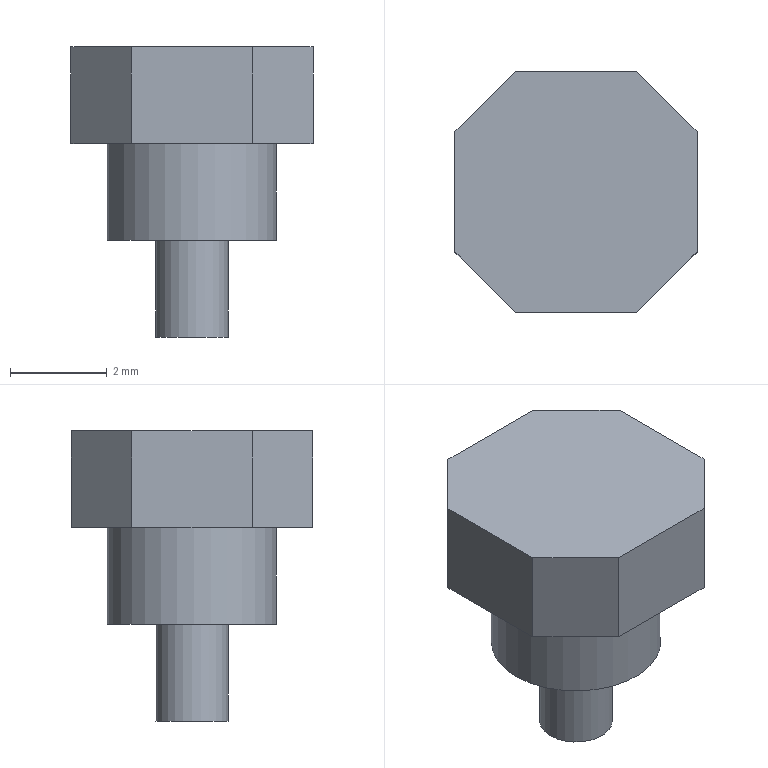Part | NX | features DATUM_CSYS 4, EXTRUDE 3, SKETCH 3, SYMBOLIC_THREAD 1 | 1 solid | 14 faces | box 5 x 4.979 x 6 mm | volume 66.325 mm3 | plane 12 | cylinder 2 | commonest cylinder face diameters 1.5 x1 3.5 x1
STEP:
#1=CARTESIAN_POINT('',(-1.251,-2.49,0.));
#2=VERTEX_POINT('',#1);
#3=CARTESIAN_POINT('',(1.251,-2.49,0.));
#4=VERTEX_POINT('',#3);
#5=CARTESIAN_POINT('',(-1.251,-2.49,0.));
#6=DIRECTION('',(1.,0.,0.));
#7=VECTOR('',#6,1000.);
#8=LINE('',#5,#7);
#9=EDGE_CURVE('',#2,#4,#8,.T.);
#10=ORIENTED_EDGE('',*,*,#9,.T.);
#11=CARTESIAN_POINT('',(1.251,-2.49,2.));
#12=VERTEX_POINT('',#11);
#13=CARTESIAN_POINT('',(1.251,-2.49,2.));
#14=DIRECTION('',(0.,0.,-1.));
#15=VECTOR('',#14,1000.);
#16=LINE('',#13,#15);
#17=EDGE_CURVE('',#12,#4,#16,.T.);
#18=ORIENTED_EDGE('',*,*,#17,.F.);
#19=CARTESIAN_POINT('',(-1.251,-2.49,2.));
#20=VERTEX_POINT('',#19);
#21=CARTESIAN_POINT('',(-1.251,-2.49,2.));
#22=DIRECTION('',(1.,0.,0.));
#23=VECTOR('',#22,1000.);
#24=LINE('',#21,#23);
#25=EDGE_CURVE('',#20,#12,#24,.T.);
#26=ORIENTED_EDGE('',*,*,#25,.F.);
#27=CARTESIAN_POINT('',(-1.251,-2.49,2.));
#28=DIRECTION('',(0.,0.,-1.));
#29=VECTOR('',#28,1000.);
#30=LINE('',#27,#29);
#31=EDGE_CURVE('',#20,#2,#30,.T.);
#32=ORIENTED_EDGE('',*,*,#31,.T.);
#33=EDGE_LOOP('',(#10,#18,#26,#32));
#34=FACE_BOUND('',#33,.T.);
#35=CARTESIAN_POINT('',(-1.251,-2.49,2.));
#36=DIRECTION('',(0.,1.,0.));
#37=DIRECTION('',(-1.,0.,0.));
#38=AXIS2_PLACEMENT_3D('',#35,#36,#37);
#39=PLANE('',#38);
#40=ADVANCED_FACE('',(#34),#39,.F.);
#41=CARTESIAN_POINT('',(2.5,-1.24,0.));
#42=VERTEX_POINT('',#41);
#43=CARTESIAN_POINT('',(1.251,-2.49,0.));
#44=DIRECTION('',(0.7071,0.7071,0.));
#45=VECTOR('',#44,1000.);
#46=LINE('',#43,#45);
#47=EDGE_CURVE('',#4,#42,#46,.T.);
#48=ORIENTED_EDGE('',*,*,#47,.T.);
#49=CARTESIAN_POINT('',(2.5,-1.24,2.));
#50=VERTEX_POINT('',#49);
#51=CARTESIAN_POINT('',(2.5,-1.24,2.));
#52=DIRECTION('',(0.,0.,-1.));
#53=VECTOR('',#52,1000.);
#54=LINE('',#51,#53);
#55=EDGE_CURVE('',#50,#42,#54,.T.);
#56=ORIENTED_EDGE('',*,*,#55,.F.);
#57=CARTESIAN_POINT('',(1.251,-2.49,2.));
#58=DIRECTION('',(0.7071,0.7071,0.));
#59=VECTOR('',#58,1000.);
#60=LINE('',#57,#59);
#61=EDGE_CURVE('',#12,#50,#60,.T.);
#62=ORIENTED_EDGE('',*,*,#61,.F.);
#63=ORIENTED_EDGE('',*,*,#17,.T.);
#64=EDGE_LOOP('',(#48,#56,#62,#63));
#65=FACE_BOUND('',#64,.T.);
#66=CARTESIAN_POINT('',(1.251,-2.49,2.));
#67=DIRECTION('',(-0.7071,0.7071,0.));
#68=DIRECTION('',(-0.7071,-0.7071,0.));
#69=AXIS2_PLACEMENT_3D('',#66,#67,#68);
#70=PLANE('',#69);
#71=ADVANCED_FACE('',(#65),#70,.F.);
#72=CARTESIAN_POINT('',(2.5,1.24,0.));
#73=VERTEX_POINT('',#72);
#74=CARTESIAN_POINT('',(2.5,-1.24,0.));
#75=DIRECTION('',(0.,1.,0.));
#76=VECTOR('',#75,1000.);
#77=LINE('',#74,#76);
#78=EDGE_CURVE('',#42,#73,#77,.T.);
#79=ORIENTED_EDGE('',*,*,#78,.T.);
#80=CARTESIAN_POINT('',(2.5,1.24,2.));
#81=VERTEX_POINT('',#80);
#82=CARTESIAN_POINT('',(2.5,1.24,2.));
#83=DIRECTION('',(0.,0.,-1.));
#84=VECTOR('',#83,1000.);
#85=LINE('',#82,#84);
#86=EDGE_CURVE('',#81,#73,#85,.T.);
#87=ORIENTED_EDGE('',*,*,#86,.F.);
#88=CARTESIAN_POINT('',(2.5,-1.24,2.));
#89=DIRECTION('',(0.,1.,0.));
#90=VECTOR('',#89,1000.);
#91=LINE('',#88,#90);
#92=EDGE_CURVE('',#50,#81,#91,.T.);
#93=ORIENTED_EDGE('',*,*,#92,.F.);
#94=ORIENTED_EDGE('',*,*,#55,.T.);
#95=EDGE_LOOP('',(#79,#87,#93,#94));
#96=FACE_BOUND('',#95,.T.);
#97=CARTESIAN_POINT('',(2.5,-1.24,2.));
#98=DIRECTION('',(-1.,0.,0.));
#99=DIRECTION('',(0.,0.,1.));
#100=AXIS2_PLACEMENT_3D('',#97,#98,#99);
#101=PLANE('',#100);
#102=ADVANCED_FACE('',(#96),#101,.F.);
#103=CARTESIAN_POINT('',(1.251,2.49,0.));
#104=VERTEX_POINT('',#103);
#105=CARTESIAN_POINT('',(2.5,1.24,0.));
#106=DIRECTION('',(-0.7071,0.7071,0.));
#107=VECTOR('',#106,1000.);
#108=LINE('',#105,#107);
#109=EDGE_CURVE('',#73,#104,#108,.T.);
#110=ORIENTED_EDGE('',*,*,#109,.T.);
#111=CARTESIAN_POINT('',(1.251,2.49,2.));
#112=VERTEX_POINT('',#111);
#113=CARTESIAN_POINT('',(1.251,2.49,2.));
#114=DIRECTION('',(0.,0.,-1.));
#115=VECTOR('',#114,1000.);
#116=LINE('',#113,#115);
#117=EDGE_CURVE('',#112,#104,#116,.T.);
#118=ORIENTED_EDGE('',*,*,#117,.F.);
#119=CARTESIAN_POINT('',(2.5,1.24,2.));
#120=DIRECTION('',(-0.7071,0.7071,0.));
#121=VECTOR('',#120,1000.);
#122=LINE('',#119,#121);
#123=EDGE_CURVE('',#81,#112,#122,.T.);
#124=ORIENTED_EDGE('',*,*,#123,.F.);
#125=ORIENTED_EDGE('',*,*,#86,.T.);
#126=EDGE_LOOP('',(#110,#118,#124,#125));
#127=FACE_BOUND('',#126,.T.);
#128=CARTESIAN_POINT('',(2.5,1.24,2.));
#129=DIRECTION('',(-0.7071,-0.7071,0.));
#130=DIRECTION('',(0.7071,-0.7071,0.));
#131=AXIS2_PLACEMENT_3D('',#128,#129,#130);
#132=PLANE('',#131);
#133=ADVANCED_FACE('',(#127),#132,.F.);
#134=CARTESIAN_POINT('',(-1.251,2.49,0.));
#135=VERTEX_POINT('',#134);
#136=CARTESIAN_POINT('',(1.251,2.49,0.));
#137=DIRECTION('',(-1.,0.,0.));
#138=VECTOR('',#137,1000.);
#139=LINE('',#136,#138);
#140=EDGE_CURVE('',#104,#135,#139,.T.);
#141=ORIENTED_EDGE('',*,*,#140,.T.);
#142=CARTESIAN_POINT('',(-1.251,2.49,2.));
#143=VERTEX_POINT('',#142);
#144=CARTESIAN_POINT('',(-1.251,2.49,2.));
#145=DIRECTION('',(0.,0.,-1.));
#146=VECTOR('',#145,1000.);
#147=LINE('',#144,#146);
#148=EDGE_CURVE('',#143,#135,#147,.T.);
#149=ORIENTED_EDGE('',*,*,#148,.F.);
#150=CARTESIAN_POINT('',(1.251,2.49,2.));
#151=DIRECTION('',(-1.,0.,0.));
#152=VECTOR('',#151,1000.);
#153=LINE('',#150,#152);
#154=EDGE_CURVE('',#112,#143,#153,.T.);
#155=ORIENTED_EDGE('',*,*,#154,.F.);
#156=ORIENTED_EDGE('',*,*,#117,.T.);
#157=EDGE_LOOP('',(#141,#149,#155,#156));
#158=FACE_BOUND('',#157,.T.);
#159=CARTESIAN_POINT('',(1.251,2.49,2.));
#160=DIRECTION('',(0.,-1.,0.));
#161=DIRECTION('',(0.,0.,-1.));
#162=AXIS2_PLACEMENT_3D('',#159,#160,#161);
#163=PLANE('',#162);
#164=ADVANCED_FACE('',(#158),#163,.F.);
#165=CARTESIAN_POINT('',(-2.5,1.24,0.));
#166=VERTEX_POINT('',#165);
#167=CARTESIAN_POINT('',(-1.251,2.49,0.));
#168=DIRECTION('',(-0.7071,-0.7071,0.));
#169=VECTOR('',#168,1000.);
#170=LINE('',#167,#169);
#171=EDGE_CURVE('',#135,#166,#170,.T.);
#172=ORIENTED_EDGE('',*,*,#171,.T.);
#173=CARTESIAN_POINT('',(-2.5,1.24,2.));
#174=VERTEX_POINT('',#173);
#175=CARTESIAN_POINT('',(-2.5,1.24,2.));
#176=DIRECTION('',(0.,0.,-1.));
#177=VECTOR('',#176,1000.);
#178=LINE('',#175,#177);
#179=EDGE_CURVE('',#174,#166,#178,.T.);
#180=ORIENTED_EDGE('',*,*,#179,.F.);
#181=CARTESIAN_POINT('',(-1.251,2.49,2.));
#182=DIRECTION('',(-0.7071,-0.7071,0.));
#183=VECTOR('',#182,1000.);
#184=LINE('',#181,#183);
#185=EDGE_CURVE('',#143,#174,#184,.T.);
#186=ORIENTED_EDGE('',*,*,#185,.F.);
#187=ORIENTED_EDGE('',*,*,#148,.T.);
#188=EDGE_LOOP('',(#172,#180,#186,#187));
#189=FACE_BOUND('',#188,.T.);
#190=CARTESIAN_POINT('',(-1.251,2.49,2.));
#191=DIRECTION('',(0.7071,-0.7071,0.));
#192=DIRECTION('',(0.7071,0.7071,0.));
#193=AXIS2_PLACEMENT_3D('',#190,#191,#192);
#194=PLANE('',#193);
#195=ADVANCED_FACE('',(#189),#194,.F.);
#196=CARTESIAN_POINT('',(-2.5,-1.24,0.));
#197=VERTEX_POINT('',#196);
#198=CARTESIAN_POINT('',(-2.5,1.24,0.));
#199=DIRECTION('',(0.,-1.,0.));
#200=VECTOR('',#199,1000.);
#201=LINE('',#198,#200);
#202=EDGE_CURVE('',#166,#197,#201,.T.);
#203=ORIENTED_EDGE('',*,*,#202,.T.);
#204=CARTESIAN_POINT('',(-2.5,-1.24,2.));
#205=VERTEX_POINT('',#204);
#206=CARTESIAN_POINT('',(-2.5,-1.24,2.));
#207=DIRECTION('',(0.,0.,-1.));
#208=VECTOR('',#207,1000.);
#209=LINE('',#206,#208);
#210=EDGE_CURVE('',#205,#197,#209,.T.);
#211=ORIENTED_EDGE('',*,*,#210,.F.);
#212=CARTESIAN_POINT('',(-2.5,1.24,2.));
#213=DIRECTION('',(0.,-1.,0.));
#214=VECTOR('',#213,1000.);
#215=LINE('',#212,#214);
#216=EDGE_CURVE('',#174,#205,#215,.T.);
#217=ORIENTED_EDGE('',*,*,#216,.F.);
#218=ORIENTED_EDGE('',*,*,#179,.T.);
#219=EDGE_LOOP('',(#203,#211,#217,#218));
#220=FACE_BOUND('',#219,.T.);
#221=CARTESIAN_POINT('',(-2.5,1.24,2.));
#222=DIRECTION('',(1.,0.,0.));
#223=DIRECTION('',(0.,0.,-1.));
#224=AXIS2_PLACEMENT_3D('',#221,#222,#223);
#225=PLANE('',#224);
#226=ADVANCED_FACE('',(#220),#225,.F.);
#227=CARTESIAN_POINT('',(-2.5,-1.24,0.));
#228=DIRECTION('',(0.7071,-0.7071,0.));
#229=VECTOR('',#228,1000.);
#230=LINE('',#227,#229);
#231=EDGE_CURVE('',#197,#2,#230,.T.);
#232=ORIENTED_EDGE('',*,*,#231,.T.);
#233=ORIENTED_EDGE('',*,*,#31,.F.);
#234=CARTESIAN_POINT('',(-2.5,-1.24,2.));
#235=DIRECTION('',(0.7071,-0.7071,0.));
#236=VECTOR('',#235,1000.);
#237=LINE('',#234,#236);
#238=EDGE_CURVE('',#205,#20,#237,.T.);
#239=ORIENTED_EDGE('',*,*,#238,.F.);
#240=ORIENTED_EDGE('',*,*,#210,.T.);
#241=EDGE_LOOP('',(#232,#233,#239,#240));
#242=FACE_BOUND('',#241,.T.);
#243=CARTESIAN_POINT('',(-2.5,-1.24,2.));
#244=DIRECTION('',(0.7071,0.7071,0.));
#245=DIRECTION('',(-0.7071,0.7071,0.));
#246=AXIS2_PLACEMENT_3D('',#243,#244,#245);
#247=PLANE('',#246);
#248=ADVANCED_FACE('',(#242),#247,.F.);
#249=ORIENTED_EDGE('',*,*,#25,.T.);
#250=ORIENTED_EDGE('',*,*,#61,.T.);
#251=ORIENTED_EDGE('',*,*,#92,.T.);
#252=ORIENTED_EDGE('',*,*,#123,.T.);
#253=ORIENTED_EDGE('',*,*,#154,.T.);
#254=ORIENTED_EDGE('',*,*,#185,.T.);
#255=ORIENTED_EDGE('',*,*,#216,.T.);
#256=ORIENTED_EDGE('',*,*,#238,.T.);
#257=EDGE_LOOP('',(#249,#250,#251,#252,#253,#254,#255,#256));
#258=FACE_BOUND('',#257,.T.);
#259=CARTESIAN_POINT('',(0.,0.,2.));
#260=DIRECTION('',(0.,0.,1.));
#261=DIRECTION('',(1.,0.,0.));
#262=AXIS2_PLACEMENT_3D('',#259,#260,#261);
#263=PLANE('',#262);
#264=ADVANCED_FACE('',(#258),#263,.T.);
#265=CARTESIAN_POINT('',(-1.237,1.237,0.));
#266=VERTEX_POINT('',#265);
#267=CARTESIAN_POINT('',(0.,0.,0.));
#268=DIRECTION('',(0.,0.,1.));
#269=DIRECTION('',(-0.7071,0.7071,0.));
#270=AXIS2_PLACEMENT_3D('',#267,#268,#269);
#271=CIRCLE('',#270,1.75);
#272=EDGE_CURVE('',#266,#266,#271,.T.);
#273=ORIENTED_EDGE('',*,*,#272,.T.);
#274=EDGE_LOOP('',(#273));
#275=FACE_BOUND('',#274,.T.);
#276=ORIENTED_EDGE('',*,*,#9,.F.);
#277=ORIENTED_EDGE('',*,*,#231,.F.);
#278=ORIENTED_EDGE('',*,*,#202,.F.);
#279=ORIENTED_EDGE('',*,*,#171,.F.);
#280=ORIENTED_EDGE('',*,*,#140,.F.);
#281=ORIENTED_EDGE('',*,*,#109,.F.);
#282=ORIENTED_EDGE('',*,*,#78,.F.);
#283=ORIENTED_EDGE('',*,*,#47,.F.);
#284=EDGE_LOOP('',(#276,#277,#278,#279,#280,#281,#282,#283));
#285=FACE_BOUND('',#284,.T.);
#286=CARTESIAN_POINT('',(0.,0.,0.));
#287=DIRECTION('',(0.,0.,1.));
#288=DIRECTION('',(1.,0.,0.));
#289=AXIS2_PLACEMENT_3D('',#286,#287,#288);
#290=PLANE('',#289);
#291=ADVANCED_FACE('',(#275,#285),#290,.F.);
#292=CARTESIAN_POINT('',(-1.237,1.237,-2.));
#293=VERTEX_POINT('',#292);
#294=CARTESIAN_POINT('',(0.,0.,-2.));
#295=DIRECTION('',(0.,0.,1.));
#296=DIRECTION('',(-0.7071,0.7071,0.));
#297=AXIS2_PLACEMENT_3D('',#294,#295,#296);
#298=CIRCLE('',#297,1.75);
#299=EDGE_CURVE('',#293,#293,#298,.T.);
#300=ORIENTED_EDGE('',*,*,#299,.T.);
#301=EDGE_LOOP('',(#300));
#302=FACE_BOUND('',#301,.T.);
#303=ORIENTED_EDGE('',*,*,#272,.F.);
#304=EDGE_LOOP('',(#303));
#305=FACE_BOUND('',#304,.T.);
#306=CARTESIAN_POINT('',(0.,0.,-2.));
#307=DIRECTION('',(0.,0.,1.));
#308=DIRECTION('',(1.,0.,0.));
#309=AXIS2_PLACEMENT_3D('',#306,#307,#308);
#310=CYLINDRICAL_SURFACE('',#309,1.75);
#311=ADVANCED_FACE('',(#302,#305),#310,.T.);
#312=CARTESIAN_POINT('',(0.75,0.,-2.));
#313=VERTEX_POINT('',#312);
#314=CARTESIAN_POINT('',(0.,0.,-2.));
#315=DIRECTION('',(0.,0.,1.));
#316=DIRECTION('',(1.,0.,0.));
#317=AXIS2_PLACEMENT_3D('',#314,#315,#316);
#318=CIRCLE('',#317,0.75);
#319=EDGE_CURVE('',#313,#313,#318,.T.);
#320=ORIENTED_EDGE('',*,*,#319,.T.);
#321=EDGE_LOOP('',(#320));
#322=FACE_BOUND('',#321,.T.);
#323=ORIENTED_EDGE('',*,*,#299,.F.);
#324=EDGE_LOOP('',(#323));
#325=FACE_BOUND('',#324,.T.);
#326=CARTESIAN_POINT('',(0.,0.,-2.));
#327=DIRECTION('',(0.,0.,1.));
#328=DIRECTION('',(1.,0.,0.));
#329=AXIS2_PLACEMENT_3D('',#326,#327,#328);
#330=PLANE('',#329);
#331=ADVANCED_FACE('',(#322,#325),#330,.F.);
#332=CARTESIAN_POINT('',(0.75,0.,-4.));
#333=VERTEX_POINT('',#332);
#334=CARTESIAN_POINT('',(0.,0.,-4.));
#335=DIRECTION('',(0.,0.,1.));
#336=DIRECTION('',(1.,0.,0.));
#337=AXIS2_PLACEMENT_3D('',#334,#335,#336);
#338=CIRCLE('',#337,0.75);
#339=EDGE_CURVE('',#333,#333,#338,.T.);
#340=ORIENTED_EDGE('',*,*,#339,.T.);
#341=EDGE_LOOP('',(#340));
#342=FACE_BOUND('',#341,.T.);
#343=ORIENTED_EDGE('',*,*,#319,.F.);
#344=EDGE_LOOP('',(#343));
#345=FACE_BOUND('',#344,.T.);
#346=CARTESIAN_POINT('',(0.,0.,-4.));
#347=DIRECTION('',(0.,0.,1.));
#348=DIRECTION('',(1.,0.,0.));
#349=AXIS2_PLACEMENT_3D('',#346,#347,#348);
#350=CYLINDRICAL_SURFACE('',#349,0.75);
#351=ADVANCED_FACE('',(#342,#345),#350,.T.);
#352=ORIENTED_EDGE('',*,*,#339,.F.);
#353=EDGE_LOOP('',(#352));
#354=FACE_BOUND('',#353,.T.);
#355=CARTESIAN_POINT('',(0.,0.,-4.));
#356=DIRECTION('',(0.,0.,1.));
#357=DIRECTION('',(1.,0.,0.));
#358=AXIS2_PLACEMENT_3D('',#355,#356,#357);
#359=PLANE('',#358);
#360=ADVANCED_FACE('',(#354),#359,.F.);
#361=CLOSED_SHELL('',(#40,#71,#102,#133,#164,#195,#226,#248,#264,#291,#311,#331,#351,#360));
#362=MANIFOLD_SOLID_BREP('',#361);
#363=(LENGTH_UNIT()NAMED_UNIT(*)SI_UNIT(.MILLI.,.METRE.));
#364=UNCERTAINTY_MEASURE_WITH_UNIT(LENGTH_MEASURE(0.00001),#363,'','');
#365=(NAMED_UNIT(*)PLANE_ANGLE_UNIT()SI_UNIT($,.RADIAN.));
#366=(NAMED_UNIT(*)SI_UNIT($,.STERADIAN.)SOLID_ANGLE_UNIT());
#367=(GEOMETRIC_REPRESENTATION_CONTEXT(3)GLOBAL_UNCERTAINTY_ASSIGNED_CONTEXT((#364))GLOBAL_UNIT_ASSIGNED_CONTEXT((#363,#365,#366))REPRESENTATION_CONTEXT('',''));
#368=ADVANCED_BREP_SHAPE_REPRESENTATION('',(#362),#367);